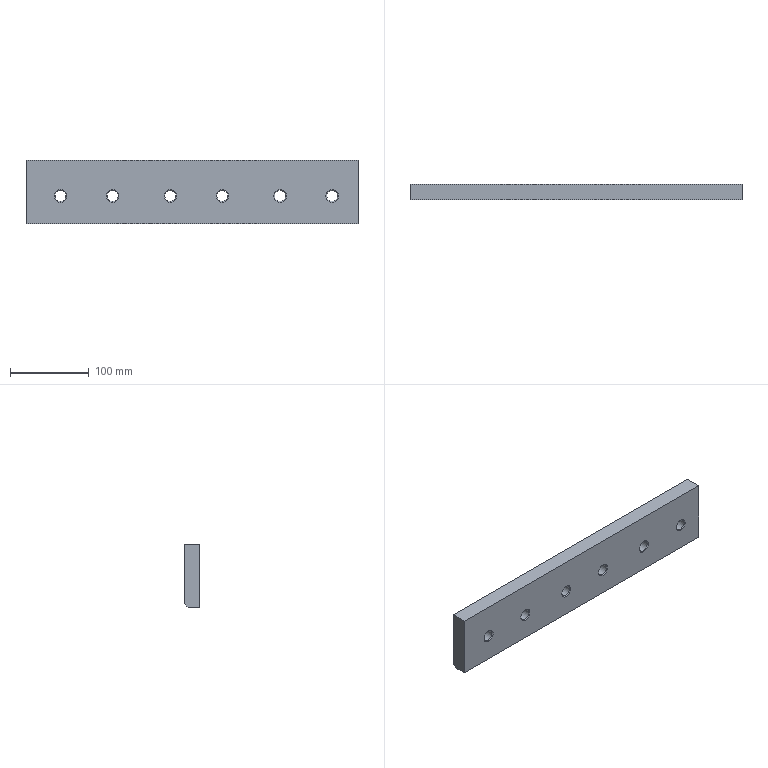Part | NX | features SIMPLE HOLE 6, SYMBOLIC_THREAD 6, DATUM_CSYS 3, SKETCH 2, CHAMFER 1, EXTRUDE 1, HOLE PACKAGE 1, LINKED_FACE 1 | 1 solid | 25 faces | box 421 x 20 x 80 mm | volume 649588 mm3 | cone 12 | plane 7 | cylinder 6 | commonest cylinder face diameters 14 x6
STEP:
#1=CARTESIAN_POINT('',(-316.,-77.,-144.));
#2=VERTEX_POINT('',#1);
#3=CARTESIAN_POINT('',(105.,-77.,-144.));
#4=VERTEX_POINT('',#3);
#5=CARTESIAN_POINT('',(-316.,-77.,-144.));
#6=DIRECTION('',(1.,0.,0.));
#7=VECTOR('',#6,1000.);
#8=LINE('',#5,#7);
#9=EDGE_CURVE('',#2,#4,#8,.T.);
#10=ORIENTED_EDGE('',*,*,#9,.T.);
#11=CARTESIAN_POINT('',(105.,-57.,-144.));
#12=VERTEX_POINT('',#11);
#13=CARTESIAN_POINT('',(105.,-57.,-144.));
#14=DIRECTION('',(0.,-1.,0.));
#15=VECTOR('',#14,1000.);
#16=LINE('',#13,#15);
#17=EDGE_CURVE('',#12,#4,#16,.T.);
#18=ORIENTED_EDGE('',*,*,#17,.F.);
#19=CARTESIAN_POINT('',(-316.,-57.,-144.));
#20=VERTEX_POINT('',#19);
#21=CARTESIAN_POINT('',(-316.,-57.,-144.));
#22=DIRECTION('',(1.,0.,0.));
#23=VECTOR('',#22,1000.);
#24=LINE('',#21,#23);
#25=EDGE_CURVE('',#20,#12,#24,.T.);
#26=ORIENTED_EDGE('',*,*,#25,.F.);
#27=CARTESIAN_POINT('',(-316.,-57.,-144.));
#28=DIRECTION('',(0.,-1.,0.));
#29=VECTOR('',#28,1000.);
#30=LINE('',#27,#29);
#31=EDGE_CURVE('',#20,#2,#30,.T.);
#32=ORIENTED_EDGE('',*,*,#31,.T.);
#33=EDGE_LOOP('',(#10,#18,#26,#32));
#34=FACE_BOUND('',#33,.T.);
#35=CARTESIAN_POINT('',(-316.,-57.,-144.));
#36=DIRECTION('',(0.,0.,-1.));
#37=DIRECTION('',(-1.,0.,0.));
#38=AXIS2_PLACEMENT_3D('',#35,#36,#37);
#39=PLANE('',#38);
#40=ADVANCED_FACE('',(#34),#39,.F.);
#41=CARTESIAN_POINT('',(105.,-62.,-224.));
#42=VERTEX_POINT('',#41);
#43=CARTESIAN_POINT('',(105.,-77.,-224.));
#44=VERTEX_POINT('',#43);
#45=CARTESIAN_POINT('',(105.,-57.,-224.));
#46=DIRECTION('',(0.,-1.,0.));
#47=VECTOR('',#46,1000.);
#48=LINE('',#45,#47);
#49=EDGE_CURVE('',#42,#44,#48,.T.);
#50=ORIENTED_EDGE('',*,*,#49,.F.);
#51=CARTESIAN_POINT('',(105.,-57.,-219.));
#52=VERTEX_POINT('',#51);
#53=CARTESIAN_POINT('',(105.,-57.,-219.));
#54=DIRECTION('',(0.,0.7071,0.7071));
#55=VECTOR('',#54,1000.);
#56=LINE('',#53,#55);
#57=EDGE_CURVE('',#42,#52,#56,.T.);
#58=ORIENTED_EDGE('',*,*,#57,.T.);
#59=CARTESIAN_POINT('',(105.,-57.,-144.));
#60=DIRECTION('',(0.,0.,-1.));
#61=VECTOR('',#60,1000.);
#62=LINE('',#59,#61);
#63=EDGE_CURVE('',#12,#52,#62,.T.);
#64=ORIENTED_EDGE('',*,*,#63,.F.);
#65=ORIENTED_EDGE('',*,*,#17,.T.);
#66=CARTESIAN_POINT('',(105.,-77.,-144.));
#67=DIRECTION('',(0.,0.,-1.));
#68=VECTOR('',#67,1000.);
#69=LINE('',#66,#68);
#70=EDGE_CURVE('',#4,#44,#69,.T.);
#71=ORIENTED_EDGE('',*,*,#70,.T.);
#72=EDGE_LOOP('',(#50,#58,#64,#65,#71));
#73=FACE_BOUND('',#72,.T.);
#74=CARTESIAN_POINT('',(105.,-57.,-144.));
#75=DIRECTION('',(-1.,0.,0.));
#76=DIRECTION('',(0.,0.,1.));
#77=AXIS2_PLACEMENT_3D('',#74,#75,#76);
#78=PLANE('',#77);
#79=ADVANCED_FACE('',(#73),#78,.F.);
#80=CARTESIAN_POINT('',(-316.,-62.,-224.));
#81=VERTEX_POINT('',#80);
#82=CARTESIAN_POINT('',(-316.,-77.,-224.));
#83=VERTEX_POINT('',#82);
#84=CARTESIAN_POINT('',(-316.,-57.,-224.));
#85=DIRECTION('',(0.,-1.,0.));
#86=VECTOR('',#85,1000.);
#87=LINE('',#84,#86);
#88=EDGE_CURVE('',#81,#83,#87,.T.);
#89=ORIENTED_EDGE('',*,*,#88,.F.);
#90=CARTESIAN_POINT('',(105.,-62.,-224.));
#91=DIRECTION('',(1.,0.,0.));
#92=VECTOR('',#91,1000.);
#93=LINE('',#90,#92);
#94=EDGE_CURVE('',#81,#42,#93,.T.);
#95=ORIENTED_EDGE('',*,*,#94,.T.);
#96=ORIENTED_EDGE('',*,*,#49,.T.);
#97=CARTESIAN_POINT('',(105.,-77.,-224.));
#98=DIRECTION('',(-1.,0.,0.));
#99=VECTOR('',#98,1000.);
#100=LINE('',#97,#99);
#101=EDGE_CURVE('',#44,#83,#100,.T.);
#102=ORIENTED_EDGE('',*,*,#101,.T.);
#103=EDGE_LOOP('',(#89,#95,#96,#102));
#104=FACE_BOUND('',#103,.T.);
#105=CARTESIAN_POINT('',(105.,-57.,-224.));
#106=DIRECTION('',(0.,0.,1.));
#107=DIRECTION('',(1.,0.,0.));
#108=AXIS2_PLACEMENT_3D('',#105,#106,#107);
#109=PLANE('',#108);
#110=ADVANCED_FACE('',(#104),#109,.F.);
#111=CARTESIAN_POINT('',(-316.,-57.,-219.));
#112=VERTEX_POINT('',#111);
#113=CARTESIAN_POINT('',(-316.,-57.,-224.));
#114=DIRECTION('',(0.,0.,1.));
#115=VECTOR('',#114,1000.);
#116=LINE('',#113,#115);
#117=EDGE_CURVE('',#112,#20,#116,.T.);
#118=ORIENTED_EDGE('',*,*,#117,.F.);
#119=CARTESIAN_POINT('',(-316.,-57.,-219.));
#120=DIRECTION('',(0.,-0.7071,-0.7071));
#121=VECTOR('',#120,1000.);
#122=LINE('',#119,#121);
#123=EDGE_CURVE('',#112,#81,#122,.T.);
#124=ORIENTED_EDGE('',*,*,#123,.T.);
#125=ORIENTED_EDGE('',*,*,#88,.T.);
#126=CARTESIAN_POINT('',(-316.,-77.,-224.));
#127=DIRECTION('',(0.,0.,1.));
#128=VECTOR('',#127,1000.);
#129=LINE('',#126,#128);
#130=EDGE_CURVE('',#83,#2,#129,.T.);
#131=ORIENTED_EDGE('',*,*,#130,.T.);
#132=ORIENTED_EDGE('',*,*,#31,.F.);
#133=EDGE_LOOP('',(#118,#124,#125,#131,#132));
#134=FACE_BOUND('',#133,.T.);
#135=CARTESIAN_POINT('',(-316.,-57.,-224.));
#136=DIRECTION('',(1.,0.,0.));
#137=DIRECTION('',(0.,0.,-1.));
#138=AXIS2_PLACEMENT_3D('',#135,#136,#137);
#139=PLANE('',#138);
#140=ADVANCED_FACE('',(#134),#139,.F.);
#141=CARTESIAN_POINT('',(72.252,-57.,-181.));
#142=VERTEX_POINT('',#141);
#143=CARTESIAN_POINT('',(72.252,-57.,-189.));
#144=DIRECTION('',(0.,1.,0.));
#145=DIRECTION('',(0.,0.,1.));
#146=AXIS2_PLACEMENT_3D('',#143,#144,#145);
#147=CIRCLE('',#146,8.);
#148=EDGE_CURVE('',#142,#142,#147,.F.);
#149=ORIENTED_EDGE('',*,*,#148,.T.);
#150=EDGE_LOOP('',(#149));
#151=FACE_BOUND('',#150,.T.);
#152=CARTESIAN_POINT('',(6.252,-57.,-181.));
#153=VERTEX_POINT('',#152);
#154=CARTESIAN_POINT('',(6.252,-57.,-189.));
#155=DIRECTION('',(0.,1.,0.));
#156=DIRECTION('',(0.,0.,1.));
#157=AXIS2_PLACEMENT_3D('',#154,#155,#156);
#158=CIRCLE('',#157,8.);
#159=EDGE_CURVE('',#153,#153,#158,.F.);
#160=ORIENTED_EDGE('',*,*,#159,.T.);
#161=EDGE_LOOP('',(#160));
#162=FACE_BOUND('',#161,.T.);
#163=CARTESIAN_POINT('',(-66.998,-57.,-181.));
#164=VERTEX_POINT('',#163);
#165=CARTESIAN_POINT('',(-66.998,-57.,-189.));
#166=DIRECTION('',(0.,1.,0.));
#167=DIRECTION('',(0.,0.,1.));
#168=AXIS2_PLACEMENT_3D('',#165,#166,#167);
#169=CIRCLE('',#168,8.);
#170=EDGE_CURVE('',#164,#164,#169,.F.);
#171=ORIENTED_EDGE('',*,*,#170,.T.);
#172=EDGE_LOOP('',(#171));
#173=FACE_BOUND('',#172,.T.);
#174=CARTESIAN_POINT('',(-132.998,-57.,-181.));
#175=VERTEX_POINT('',#174);
#176=CARTESIAN_POINT('',(-132.998,-57.,-189.));
#177=DIRECTION('',(0.,1.,0.));
#178=DIRECTION('',(0.,0.,1.));
#179=AXIS2_PLACEMENT_3D('',#176,#177,#178);
#180=CIRCLE('',#179,8.);
#181=EDGE_CURVE('',#175,#175,#180,.F.);
#182=ORIENTED_EDGE('',*,*,#181,.T.);
#183=EDGE_LOOP('',(#182));
#184=FACE_BOUND('',#183,.T.);
#185=CARTESIAN_POINT('',(-206.248,-57.,-181.));
#186=VERTEX_POINT('',#185);
#187=CARTESIAN_POINT('',(-206.248,-57.,-189.));
#188=DIRECTION('',(0.,1.,0.));
#189=DIRECTION('',(0.,0.,1.));
#190=AXIS2_PLACEMENT_3D('',#187,#188,#189);
#191=CIRCLE('',#190,8.);
#192=EDGE_CURVE('',#186,#186,#191,.F.);
#193=ORIENTED_EDGE('',*,*,#192,.T.);
#194=EDGE_LOOP('',(#193));
#195=FACE_BOUND('',#194,.T.);
#196=CARTESIAN_POINT('',(-272.248,-57.,-181.));
#197=VERTEX_POINT('',#196);
#198=CARTESIAN_POINT('',(-272.248,-57.,-189.));
#199=DIRECTION('',(0.,1.,0.));
#200=DIRECTION('',(0.,0.,1.));
#201=AXIS2_PLACEMENT_3D('',#198,#199,#200);
#202=CIRCLE('',#201,8.);
#203=EDGE_CURVE('',#197,#197,#202,.F.);
#204=ORIENTED_EDGE('',*,*,#203,.T.);
#205=EDGE_LOOP('',(#204));
#206=FACE_BOUND('',#205,.T.);
#207=ORIENTED_EDGE('',*,*,#63,.T.);
#208=CARTESIAN_POINT('',(-316.,-57.,-219.));
#209=DIRECTION('',(-1.,0.,0.));
#210=VECTOR('',#209,1000.);
#211=LINE('',#208,#210);
#212=EDGE_CURVE('',#52,#112,#211,.T.);
#213=ORIENTED_EDGE('',*,*,#212,.T.);
#214=ORIENTED_EDGE('',*,*,#117,.T.);
#215=ORIENTED_EDGE('',*,*,#25,.T.);
#216=EDGE_LOOP('',(#207,#213,#214,#215));
#217=FACE_BOUND('',#216,.T.);
#218=CARTESIAN_POINT('',(0.,-57.,0.));
#219=DIRECTION('',(0.,1.,0.));
#220=DIRECTION('',(0.,0.,1.));
#221=AXIS2_PLACEMENT_3D('',#218,#219,#220);
#222=PLANE('',#221);
#223=ADVANCED_FACE('',(#151,#162,#173,#184,#195,#206,#217),#222,.T.);
#224=CARTESIAN_POINT('',(72.252,-77.,-181.));
#225=VERTEX_POINT('',#224);
#226=CARTESIAN_POINT('',(72.252,-77.,-189.));
#227=DIRECTION('',(0.,1.,0.));
#228=DIRECTION('',(0.,0.,1.));
#229=AXIS2_PLACEMENT_3D('',#226,#227,#228);
#230=CIRCLE('',#229,8.);
#231=EDGE_CURVE('',#225,#225,#230,.T.);
#232=ORIENTED_EDGE('',*,*,#231,.T.);
#233=EDGE_LOOP('',(#232));
#234=FACE_BOUND('',#233,.T.);
#235=CARTESIAN_POINT('',(6.252,-77.,-181.));
#236=VERTEX_POINT('',#235);
#237=CARTESIAN_POINT('',(6.252,-77.,-189.));
#238=DIRECTION('',(0.,1.,0.));
#239=DIRECTION('',(0.,0.,1.));
#240=AXIS2_PLACEMENT_3D('',#237,#238,#239);
#241=CIRCLE('',#240,8.);
#242=EDGE_CURVE('',#236,#236,#241,.T.);
#243=ORIENTED_EDGE('',*,*,#242,.T.);
#244=EDGE_LOOP('',(#243));
#245=FACE_BOUND('',#244,.T.);
#246=CARTESIAN_POINT('',(-66.998,-77.,-181.));
#247=VERTEX_POINT('',#246);
#248=CARTESIAN_POINT('',(-66.998,-77.,-189.));
#249=DIRECTION('',(0.,1.,0.));
#250=DIRECTION('',(0.,0.,1.));
#251=AXIS2_PLACEMENT_3D('',#248,#249,#250);
#252=CIRCLE('',#251,8.);
#253=EDGE_CURVE('',#247,#247,#252,.T.);
#254=ORIENTED_EDGE('',*,*,#253,.T.);
#255=EDGE_LOOP('',(#254));
#256=FACE_BOUND('',#255,.T.);
#257=CARTESIAN_POINT('',(-132.998,-77.,-181.));
#258=VERTEX_POINT('',#257);
#259=CARTESIAN_POINT('',(-132.998,-77.,-189.));
#260=DIRECTION('',(0.,1.,0.));
#261=DIRECTION('',(0.,0.,1.));
#262=AXIS2_PLACEMENT_3D('',#259,#260,#261);
#263=CIRCLE('',#262,8.);
#264=EDGE_CURVE('',#258,#258,#263,.T.);
#265=ORIENTED_EDGE('',*,*,#264,.T.);
#266=EDGE_LOOP('',(#265));
#267=FACE_BOUND('',#266,.T.);
#268=CARTESIAN_POINT('',(-206.248,-77.,-181.));
#269=VERTEX_POINT('',#268);
#270=CARTESIAN_POINT('',(-206.248,-77.,-189.));
#271=DIRECTION('',(0.,1.,0.));
#272=DIRECTION('',(0.,0.,1.));
#273=AXIS2_PLACEMENT_3D('',#270,#271,#272);
#274=CIRCLE('',#273,8.);
#275=EDGE_CURVE('',#269,#269,#274,.T.);
#276=ORIENTED_EDGE('',*,*,#275,.T.);
#277=EDGE_LOOP('',(#276));
#278=FACE_BOUND('',#277,.T.);
#279=CARTESIAN_POINT('',(-272.248,-77.,-181.));
#280=VERTEX_POINT('',#279);
#281=CARTESIAN_POINT('',(-272.248,-77.,-189.));
#282=DIRECTION('',(0.,1.,0.));
#283=DIRECTION('',(0.,0.,1.));
#284=AXIS2_PLACEMENT_3D('',#281,#282,#283);
#285=CIRCLE('',#284,8.);
#286=EDGE_CURVE('',#280,#280,#285,.T.);
#287=ORIENTED_EDGE('',*,*,#286,.T.);
#288=EDGE_LOOP('',(#287));
#289=FACE_BOUND('',#288,.T.);
#290=ORIENTED_EDGE('',*,*,#9,.F.);
#291=ORIENTED_EDGE('',*,*,#130,.F.);
#292=ORIENTED_EDGE('',*,*,#101,.F.);
#293=ORIENTED_EDGE('',*,*,#70,.F.);
#294=EDGE_LOOP('',(#290,#291,#292,#293));
#295=FACE_BOUND('',#294,.T.);
#296=CARTESIAN_POINT('',(0.,-77.,0.));
#297=DIRECTION('',(0.,1.,0.));
#298=DIRECTION('',(0.,0.,1.));
#299=AXIS2_PLACEMENT_3D('',#296,#297,#298);
#300=PLANE('',#299);
#301=ADVANCED_FACE('',(#234,#245,#256,#267,#278,#289,#295),#300,.F.);
#302=ORIENTED_EDGE('',*,*,#57,.F.);
#303=ORIENTED_EDGE('',*,*,#94,.F.);
#304=ORIENTED_EDGE('',*,*,#123,.F.);
#305=ORIENTED_EDGE('',*,*,#212,.F.);
#306=EDGE_LOOP('',(#302,#303,#304,#305));
#307=FACE_BOUND('',#306,.T.);
#308=CARTESIAN_POINT('',(0.,-57.,-219.));
#309=DIRECTION('',(0.,0.7071,-0.7071));
#310=DIRECTION('',(1.,0.,0.));
#311=AXIS2_PLACEMENT_3D('',#308,#309,#310);
#312=PLANE('',#311);
#313=ADVANCED_FACE('',(#307),#312,.T.);
#314=CARTESIAN_POINT('',(-272.248,-58.,-182.));
#315=VERTEX_POINT('',#314);
#316=CARTESIAN_POINT('',(-272.248,-58.,-189.));
#317=DIRECTION('',(0.,1.,0.));
#318=DIRECTION('',(0.,0.,1.));
#319=AXIS2_PLACEMENT_3D('',#316,#317,#318);
#320=CIRCLE('',#319,7.);
#321=EDGE_CURVE('',#315,#315,#320,.T.);
#322=ORIENTED_EDGE('',*,*,#321,.T.);
#323=EDGE_LOOP('',(#322));
#324=FACE_BOUND('',#323,.T.);
#325=CARTESIAN_POINT('',(-272.248,-76.,-182.));
#326=VERTEX_POINT('',#325);
#327=CARTESIAN_POINT('',(-272.248,-76.,-189.));
#328=DIRECTION('',(0.,1.,0.));
#329=DIRECTION('',(0.,0.,1.));
#330=AXIS2_PLACEMENT_3D('',#327,#328,#329);
#331=CIRCLE('',#330,7.);
#332=EDGE_CURVE('',#326,#326,#331,.F.);
#333=ORIENTED_EDGE('',*,*,#332,.T.);
#334=EDGE_LOOP('',(#333));
#335=FACE_BOUND('',#334,.T.);
#336=CARTESIAN_POINT('',(-272.248,-77.,-189.));
#337=DIRECTION('',(0.,1.,0.));
#338=DIRECTION('',(0.,0.,1.));
#339=AXIS2_PLACEMENT_3D('',#336,#337,#338);
#340=CYLINDRICAL_SURFACE('',#339,7.);
#341=ADVANCED_FACE('',(#324,#335),#340,.F.);
#342=ORIENTED_EDGE('',*,*,#332,.F.);
#343=EDGE_LOOP('',(#342));
#344=FACE_BOUND('',#343,.T.);
#345=ORIENTED_EDGE('',*,*,#286,.F.);
#346=EDGE_LOOP('',(#345));
#347=FACE_BOUND('',#346,.T.);
#348=CARTESIAN_POINT('',(-272.248,-77.,-189.));
#349=DIRECTION('',(0.,-1.,0.));
#350=DIRECTION('',(0.,0.,-1.));
#351=AXIS2_PLACEMENT_3D('',#348,#349,#350);
#352=CONICAL_SURFACE('',#351,8.,0.7854);
#353=ADVANCED_FACE('',(#344,#347),#352,.F.);
#354=ORIENTED_EDGE('',*,*,#203,.F.);
#355=EDGE_LOOP('',(#354));
#356=FACE_BOUND('',#355,.T.);
#357=ORIENTED_EDGE('',*,*,#321,.F.);
#358=EDGE_LOOP('',(#357));
#359=FACE_BOUND('',#358,.T.);
#360=CARTESIAN_POINT('',(-272.248,-58.,-189.));
#361=DIRECTION('',(0.,1.,0.));
#362=DIRECTION('',(0.,0.,1.));
#363=AXIS2_PLACEMENT_3D('',#360,#361,#362);
#364=CONICAL_SURFACE('',#363,7.,0.7854);
#365=ADVANCED_FACE('',(#356,#359),#364,.F.);
#366=CARTESIAN_POINT('',(-206.248,-58.,-182.));
#367=VERTEX_POINT('',#366);
#368=CARTESIAN_POINT('',(-206.248,-58.,-189.));
#369=DIRECTION('',(0.,1.,0.));
#370=DIRECTION('',(0.,0.,1.));
#371=AXIS2_PLACEMENT_3D('',#368,#369,#370);
#372=CIRCLE('',#371,7.);
#373=EDGE_CURVE('',#367,#367,#372,.T.);
#374=ORIENTED_EDGE('',*,*,#373,.T.);
#375=EDGE_LOOP('',(#374));
#376=FACE_BOUND('',#375,.T.);
#377=CARTESIAN_POINT('',(-206.248,-76.,-182.));
#378=VERTEX_POINT('',#377);
#379=CARTESIAN_POINT('',(-206.248,-76.,-189.));
#380=DIRECTION('',(0.,1.,0.));
#381=DIRECTION('',(0.,0.,1.));
#382=AXIS2_PLACEMENT_3D('',#379,#380,#381);
#383=CIRCLE('',#382,7.);
#384=EDGE_CURVE('',#378,#378,#383,.F.);
#385=ORIENTED_EDGE('',*,*,#384,.T.);
#386=EDGE_LOOP('',(#385));
#387=FACE_BOUND('',#386,.T.);
#388=CARTESIAN_POINT('',(-206.248,-77.,-189.));
#389=DIRECTION('',(0.,1.,0.));
#390=DIRECTION('',(0.,0.,1.));
#391=AXIS2_PLACEMENT_3D('',#388,#389,#390);
#392=CYLINDRICAL_SURFACE('',#391,7.);
#393=ADVANCED_FACE('',(#376,#387),#392,.F.);
#394=ORIENTED_EDGE('',*,*,#384,.F.);
#395=EDGE_LOOP('',(#394));
#396=FACE_BOUND('',#395,.T.);
#397=ORIENTED_EDGE('',*,*,#275,.F.);
#398=EDGE_LOOP('',(#397));
#399=FACE_BOUND('',#398,.T.);
#400=CARTESIAN_POINT('',(-206.248,-77.,-189.));
#401=DIRECTION('',(0.,-1.,0.));
#402=DIRECTION('',(0.,0.,-1.));
#403=AXIS2_PLACEMENT_3D('',#400,#401,#402);
#404=CONICAL_SURFACE('',#403,8.,0.7854);
#405=ADVANCED_FACE('',(#396,#399),#404,.F.);
#406=ORIENTED_EDGE('',*,*,#192,.F.);
#407=EDGE_LOOP('',(#406));
#408=FACE_BOUND('',#407,.T.);
#409=ORIENTED_EDGE('',*,*,#373,.F.);
#410=EDGE_LOOP('',(#409));
#411=FACE_BOUND('',#410,.T.);
#412=CARTESIAN_POINT('',(-206.248,-58.,-189.));
#413=DIRECTION('',(0.,1.,0.));
#414=DIRECTION('',(0.,0.,1.));
#415=AXIS2_PLACEMENT_3D('',#412,#413,#414);
#416=CONICAL_SURFACE('',#415,7.,0.7854);
#417=ADVANCED_FACE('',(#408,#411),#416,.F.);
#418=CARTESIAN_POINT('',(-132.998,-58.,-182.));
#419=VERTEX_POINT('',#418);
#420=CARTESIAN_POINT('',(-132.998,-58.,-189.));
#421=DIRECTION('',(0.,1.,0.));
#422=DIRECTION('',(0.,0.,1.));
#423=AXIS2_PLACEMENT_3D('',#420,#421,#422);
#424=CIRCLE('',#423,7.);
#425=EDGE_CURVE('',#419,#419,#424,.T.);
#426=ORIENTED_EDGE('',*,*,#425,.T.);
#427=EDGE_LOOP('',(#426));
#428=FACE_BOUND('',#427,.T.);
#429=CARTESIAN_POINT('',(-132.998,-76.,-182.));
#430=VERTEX_POINT('',#429);
#431=CARTESIAN_POINT('',(-132.998,-76.,-189.));
#432=DIRECTION('',(0.,1.,0.));
#433=DIRECTION('',(0.,0.,1.));
#434=AXIS2_PLACEMENT_3D('',#431,#432,#433);
#435=CIRCLE('',#434,7.);
#436=EDGE_CURVE('',#430,#430,#435,.F.);
#437=ORIENTED_EDGE('',*,*,#436,.T.);
#438=EDGE_LOOP('',(#437));
#439=FACE_BOUND('',#438,.T.);
#440=CARTESIAN_POINT('',(-132.998,-77.,-189.));
#441=DIRECTION('',(0.,1.,0.));
#442=DIRECTION('',(0.,0.,1.));
#443=AXIS2_PLACEMENT_3D('',#440,#441,#442);
#444=CYLINDRICAL_SURFACE('',#443,7.);
#445=ADVANCED_FACE('',(#428,#439),#444,.F.);
#446=ORIENTED_EDGE('',*,*,#436,.F.);
#447=EDGE_LOOP('',(#446));
#448=FACE_BOUND('',#447,.T.);
#449=ORIENTED_EDGE('',*,*,#264,.F.);
#450=EDGE_LOOP('',(#449));
#451=FACE_BOUND('',#450,.T.);
#452=CARTESIAN_POINT('',(-132.998,-77.,-189.));
#453=DIRECTION('',(0.,-1.,0.));
#454=DIRECTION('',(0.,0.,-1.));
#455=AXIS2_PLACEMENT_3D('',#452,#453,#454);
#456=CONICAL_SURFACE('',#455,8.,0.7854);
#457=ADVANCED_FACE('',(#448,#451),#456,.F.);
#458=ORIENTED_EDGE('',*,*,#181,.F.);
#459=EDGE_LOOP('',(#458));
#460=FACE_BOUND('',#459,.T.);
#461=ORIENTED_EDGE('',*,*,#425,.F.);
#462=EDGE_LOOP('',(#461));
#463=FACE_BOUND('',#462,.T.);
#464=CARTESIAN_POINT('',(-132.998,-58.,-189.));
#465=DIRECTION('',(0.,1.,0.));
#466=DIRECTION('',(0.,0.,1.));
#467=AXIS2_PLACEMENT_3D('',#464,#465,#466);
#468=CONICAL_SURFACE('',#467,7.,0.7854);
#469=ADVANCED_FACE('',(#460,#463),#468,.F.);
#470=CARTESIAN_POINT('',(-66.998,-58.,-182.));
#471=VERTEX_POINT('',#470);
#472=CARTESIAN_POINT('',(-66.998,-58.,-189.));
#473=DIRECTION('',(0.,1.,0.));
#474=DIRECTION('',(0.,0.,1.));
#475=AXIS2_PLACEMENT_3D('',#472,#473,#474);
#476=CIRCLE('',#475,7.);
#477=EDGE_CURVE('',#471,#471,#476,.T.);
#478=ORIENTED_EDGE('',*,*,#477,.T.);
#479=EDGE_LOOP('',(#478));
#480=FACE_BOUND('',#479,.T.);
#481=CARTESIAN_POINT('',(-66.998,-76.,-182.));
#482=VERTEX_POINT('',#481);
#483=CARTESIAN_POINT('',(-66.998,-76.,-189.));
#484=DIRECTION('',(0.,1.,0.));
#485=DIRECTION('',(0.,0.,1.));
#486=AXIS2_PLACEMENT_3D('',#483,#484,#485);
#487=CIRCLE('',#486,7.);
#488=EDGE_CURVE('',#482,#482,#487,.F.);
#489=ORIENTED_EDGE('',*,*,#488,.T.);
#490=EDGE_LOOP('',(#489));
#491=FACE_BOUND('',#490,.T.);
#492=CARTESIAN_POINT('',(-66.998,-77.,-189.));
#493=DIRECTION('',(0.,1.,0.));
#494=DIRECTION('',(0.,0.,1.));
#495=AXIS2_PLACEMENT_3D('',#492,#493,#494);
#496=CYLINDRICAL_SURFACE('',#495,7.);
#497=ADVANCED_FACE('',(#480,#491),#496,.F.);
#498=ORIENTED_EDGE('',*,*,#488,.F.);
#499=EDGE_LOOP('',(#498));
#500=FACE_BOUND('',#499,.T.);
#501=ORIENTED_EDGE('',*,*,#253,.F.);
#502=EDGE_LOOP('',(#501));
#503=FACE_BOUND('',#502,.T.);
#504=CARTESIAN_POINT('',(-66.998,-77.,-189.));
#505=DIRECTION('',(0.,-1.,0.));
#506=DIRECTION('',(0.,0.,-1.));
#507=AXIS2_PLACEMENT_3D('',#504,#505,#506);
#508=CONICAL_SURFACE('',#507,8.,0.7854);
#509=ADVANCED_FACE('',(#500,#503),#508,.F.);
#510=ORIENTED_EDGE('',*,*,#170,.F.);
#511=EDGE_LOOP('',(#510));
#512=FACE_BOUND('',#511,.T.);
#513=ORIENTED_EDGE('',*,*,#477,.F.);
#514=EDGE_LOOP('',(#513));
#515=FACE_BOUND('',#514,.T.);
#516=CARTESIAN_POINT('',(-66.998,-58.,-189.));
#517=DIRECTION('',(0.,1.,0.));
#518=DIRECTION('',(0.,0.,1.));
#519=AXIS2_PLACEMENT_3D('',#516,#517,#518);
#520=CONICAL_SURFACE('',#519,7.,0.7854);
#521=ADVANCED_FACE('',(#512,#515),#520,.F.);
#522=CARTESIAN_POINT('',(6.252,-58.,-182.));
#523=VERTEX_POINT('',#522);
#524=CARTESIAN_POINT('',(6.252,-58.,-189.));
#525=DIRECTION('',(0.,1.,0.));
#526=DIRECTION('',(0.,0.,1.));
#527=AXIS2_PLACEMENT_3D('',#524,#525,#526);
#528=CIRCLE('',#527,7.);
#529=EDGE_CURVE('',#523,#523,#528,.T.);
#530=ORIENTED_EDGE('',*,*,#529,.T.);
#531=EDGE_LOOP('',(#530));
#532=FACE_BOUND('',#531,.T.);
#533=CARTESIAN_POINT('',(6.252,-76.,-182.));
#534=VERTEX_POINT('',#533);
#535=CARTESIAN_POINT('',(6.252,-76.,-189.));
#536=DIRECTION('',(0.,1.,0.));
#537=DIRECTION('',(0.,0.,1.));
#538=AXIS2_PLACEMENT_3D('',#535,#536,#537);
#539=CIRCLE('',#538,7.);
#540=EDGE_CURVE('',#534,#534,#539,.F.);
#541=ORIENTED_EDGE('',*,*,#540,.T.);
#542=EDGE_LOOP('',(#541));
#543=FACE_BOUND('',#542,.T.);
#544=CARTESIAN_POINT('',(6.252,-77.,-189.));
#545=DIRECTION('',(0.,1.,0.));
#546=DIRECTION('',(0.,0.,1.));
#547=AXIS2_PLACEMENT_3D('',#544,#545,#546);
#548=CYLINDRICAL_SURFACE('',#547,7.);
#549=ADVANCED_FACE('',(#532,#543),#548,.F.);
#550=ORIENTED_EDGE('',*,*,#540,.F.);
#551=EDGE_LOOP('',(#550));
#552=FACE_BOUND('',#551,.T.);
#553=ORIENTED_EDGE('',*,*,#242,.F.);
#554=EDGE_LOOP('',(#553));
#555=FACE_BOUND('',#554,.T.);
#556=CARTESIAN_POINT('',(6.252,-77.,-189.));
#557=DIRECTION('',(0.,-1.,0.));
#558=DIRECTION('',(0.,0.,-1.));
#559=AXIS2_PLACEMENT_3D('',#556,#557,#558);
#560=CONICAL_SURFACE('',#559,8.,0.7854);
#561=ADVANCED_FACE('',(#552,#555),#560,.F.);
#562=ORIENTED_EDGE('',*,*,#159,.F.);
#563=EDGE_LOOP('',(#562));
#564=FACE_BOUND('',#563,.T.);
#565=ORIENTED_EDGE('',*,*,#529,.F.);
#566=EDGE_LOOP('',(#565));
#567=FACE_BOUND('',#566,.T.);
#568=CARTESIAN_POINT('',(6.252,-58.,-189.));
#569=DIRECTION('',(0.,1.,0.));
#570=DIRECTION('',(0.,0.,1.));
#571=AXIS2_PLACEMENT_3D('',#568,#569,#570);
#572=CONICAL_SURFACE('',#571,7.,0.7854);
#573=ADVANCED_FACE('',(#564,#567),#572,.F.);
#574=CARTESIAN_POINT('',(72.252,-58.,-182.));
#575=VERTEX_POINT('',#574);
#576=CARTESIAN_POINT('',(72.252,-58.,-189.));
#577=DIRECTION('',(0.,1.,0.));
#578=DIRECTION('',(0.,0.,1.));
#579=AXIS2_PLACEMENT_3D('',#576,#577,#578);
#580=CIRCLE('',#579,7.);
#581=EDGE_CURVE('',#575,#575,#580,.T.);
#582=ORIENTED_EDGE('',*,*,#581,.T.);
#583=EDGE_LOOP('',(#582));
#584=FACE_BOUND('',#583,.T.);
#585=CARTESIAN_POINT('',(72.252,-76.,-182.));
#586=VERTEX_POINT('',#585);
#587=CARTESIAN_POINT('',(72.252,-76.,-189.));
#588=DIRECTION('',(0.,1.,0.));
#589=DIRECTION('',(0.,0.,1.));
#590=AXIS2_PLACEMENT_3D('',#587,#588,#589);
#591=CIRCLE('',#590,7.);
#592=EDGE_CURVE('',#586,#586,#591,.F.);
#593=ORIENTED_EDGE('',*,*,#592,.T.);
#594=EDGE_LOOP('',(#593));
#595=FACE_BOUND('',#594,.T.);
#596=CARTESIAN_POINT('',(72.252,-77.,-189.));
#597=DIRECTION('',(0.,1.,0.));
#598=DIRECTION('',(0.,0.,1.));
#599=AXIS2_PLACEMENT_3D('',#596,#597,#598);
#600=CYLINDRICAL_SURFACE('',#599,7.);
#601=ADVANCED_FACE('',(#584,#595),#600,.F.);
#602=ORIENTED_EDGE('',*,*,#592,.F.);
#603=EDGE_LOOP('',(#602));
#604=FACE_BOUND('',#603,.T.);
#605=ORIENTED_EDGE('',*,*,#231,.F.);
#606=EDGE_LOOP('',(#605));
#607=FACE_BOUND('',#606,.T.);
#608=CARTESIAN_POINT('',(72.252,-77.,-189.));
#609=DIRECTION('',(0.,-1.,0.));
#610=DIRECTION('',(0.,0.,-1.));
#611=AXIS2_PLACEMENT_3D('',#608,#609,#610);
#612=CONICAL_SURFACE('',#611,8.,0.7854);
#613=ADVANCED_FACE('',(#604,#607),#612,.F.);
#614=ORIENTED_EDGE('',*,*,#148,.F.);
#615=EDGE_LOOP('',(#614));
#616=FACE_BOUND('',#615,.T.);
#617=ORIENTED_EDGE('',*,*,#581,.F.);
#618=EDGE_LOOP('',(#617));
#619=FACE_BOUND('',#618,.T.);
#620=CARTESIAN_POINT('',(72.252,-58.,-189.));
#621=DIRECTION('',(0.,1.,0.));
#622=DIRECTION('',(0.,0.,1.));
#623=AXIS2_PLACEMENT_3D('',#620,#621,#622);
#624=CONICAL_SURFACE('',#623,7.,0.7854);
#625=ADVANCED_FACE('',(#616,#619),#624,.F.);
#626=CLOSED_SHELL('',(#40,#79,#110,#140,#223,#301,#313,#341,#353,#365,#393,#405,#417,#445,#457,#469,#497,#509,#521,#549,#561,#573,#601,#613,#625));
#627=MANIFOLD_SOLID_BREP('',#626);
#628=(LENGTH_UNIT()NAMED_UNIT(*)SI_UNIT(.MILLI.,.METRE.));
#629=UNCERTAINTY_MEASURE_WITH_UNIT(LENGTH_MEASURE(0.00001),#628,'','');
#630=(NAMED_UNIT(*)PLANE_ANGLE_UNIT()SI_UNIT($,.RADIAN.));
#631=(NAMED_UNIT(*)SI_UNIT($,.STERADIAN.)SOLID_ANGLE_UNIT());
#632=(GEOMETRIC_REPRESENTATION_CONTEXT(3)GLOBAL_UNCERTAINTY_ASSIGNED_CONTEXT((#629))GLOBAL_UNIT_ASSIGNED_CONTEXT((#628,#630,#631))REPRESENTATION_CONTEXT('',''));
#633=ADVANCED_BREP_SHAPE_REPRESENTATION('',(#627),#632);